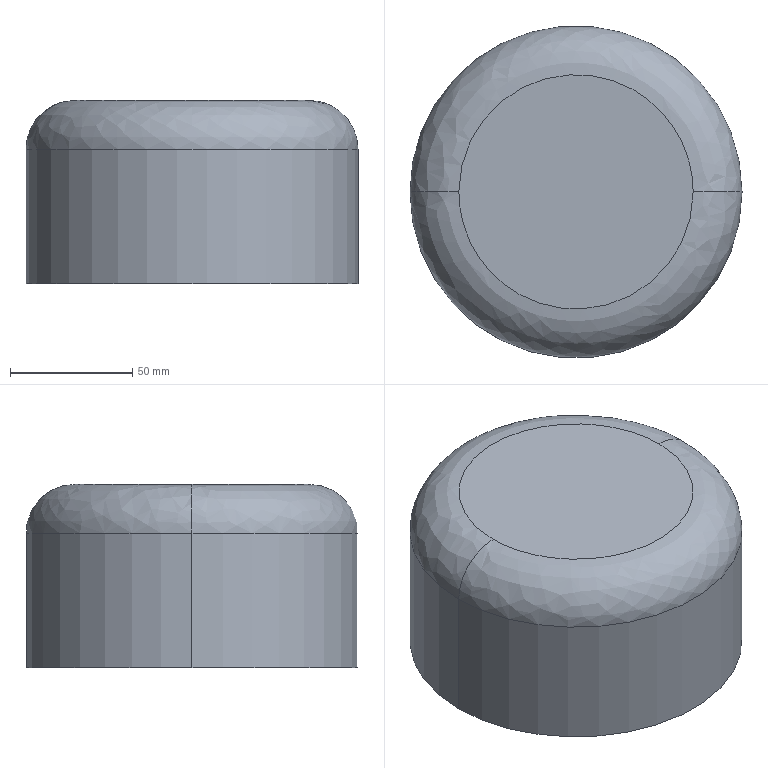Part | SolidWorks | features BaseBody 1 | 1 solid | 11 faces | box 136 x 136 x 75 mm | volume 33898 mm3 | spline 4 | cylinder 4 | plane 3 | commonest cylinder face diameters 134.4 x2 136 x2
STEP:
#1=CARTESIAN_POINT('',(48.,0.,75.));
#2=VERTEX_POINT('',#1);
#3=CARTESIAN_POINT('',(-48.,0.,75.));
#4=VERTEX_POINT('',#3);
#5=CARTESIAN_POINT('',(48.,0.,75.));
#6=CARTESIAN_POINT('',(48.,-96.,75.));
#7=CARTESIAN_POINT('',(-48.,-96.,75.));
#8=CARTESIAN_POINT('',(-48.,0.,75.));
#9=(BOUNDED_CURVE()B_SPLINE_CURVE(3,(#5,#6,#7,#8),.UNSPECIFIED.,.F.,.F.)B_SPLINE_CURVE_WITH_KNOTS((4,4),(0.,0.5),.UNSPECIFIED.)CURVE()GEOMETRIC_REPRESENTATION_ITEM()RATIONAL_B_SPLINE_CURVE((1.,0.3333,0.3333,1.))REPRESENTATION_ITEM(''));
#10=EDGE_CURVE('',#2,#4,#9,.T.);
#11=ORIENTED_EDGE('',*,*,#10,.T.);
#12=CARTESIAN_POINT('',(-68.,0.,55.));
#13=VERTEX_POINT('',#12);
#14=CARTESIAN_POINT('',(-48.,0.,55.));
#15=DIRECTION('',(0.,-1.,0.));
#16=DIRECTION('',(-1.,0.,0.));
#17=AXIS2_PLACEMENT_3D('',#14,#15,#16);
#18=CIRCLE('',#17,20.);
#19=EDGE_CURVE('',#4,#13,#18,.T.);
#20=ORIENTED_EDGE('',*,*,#19,.T.);
#21=CARTESIAN_POINT('',(68.,0.,55.));
#22=VERTEX_POINT('',#21);
#23=CARTESIAN_POINT('',(0.,0.,55.));
#24=DIRECTION('',(0.,0.,-1.));
#25=DIRECTION('',(-1.,0.,0.));
#26=AXIS2_PLACEMENT_3D('',#23,#24,#25);
#27=CIRCLE('',#26,68.);
#28=EDGE_CURVE('',#22,#13,#27,.T.);
#29=ORIENTED_EDGE('',*,*,#28,.F.);
#30=CARTESIAN_POINT('',(48.,0.,55.));
#31=DIRECTION('',(0.,1.,0.));
#32=DIRECTION('',(1.,0.,0.));
#33=AXIS2_PLACEMENT_3D('',#30,#31,#32);
#34=CIRCLE('',#33,20.);
#35=EDGE_CURVE('',#2,#22,#34,.T.);
#36=ORIENTED_EDGE('',*,*,#35,.F.);
#37=EDGE_LOOP('',(#11,#20,#29,#36));
#38=FACE_OUTER_BOUND('',#37,.T.);
#39=CARTESIAN_POINT('',(-48.,0.,75.));
#40=CARTESIAN_POINT('',(-48.,-96.,75.));
#41=CARTESIAN_POINT('',(48.,-96.,75.));
#42=CARTESIAN_POINT('',(48.,0.,75.));
#43=CARTESIAN_POINT('',(-59.716,0.,75.));
#44=CARTESIAN_POINT('',(-59.716,-119.431,75.));
#45=CARTESIAN_POINT('',(59.716,-119.431,75.));
#46=CARTESIAN_POINT('',(59.716,0.,75.));
#47=CARTESIAN_POINT('',(-68.,0.,66.716));
#48=CARTESIAN_POINT('',(-68.,-136.,66.716));
#49=CARTESIAN_POINT('',(68.,-136.,66.716));
#50=CARTESIAN_POINT('',(68.,0.,66.716));
#51=CARTESIAN_POINT('',(-68.,0.,55.));
#52=CARTESIAN_POINT('',(-68.,-136.,55.));
#53=CARTESIAN_POINT('',(68.,-136.,55.));
#54=CARTESIAN_POINT('',(68.,0.,55.));
#55=(BOUNDED_SURFACE()B_SPLINE_SURFACE(3,3,((#39,#40,#41,#42),(#43,#44,#45,#46),(#47,#48,#49,#50),(#51,#52,#53,#54)),.UNSPECIFIED.,.F.,.F.,.F.)B_SPLINE_SURFACE_WITH_KNOTS((4,4),(4,4),(0.,1.),(0.,1.),.UNSPECIFIED.)GEOMETRIC_REPRESENTATION_ITEM()RATIONAL_B_SPLINE_SURFACE(((1.,0.3333,0.3333,1.),(0.8047,0.2682,0.2682,0.8047),(0.8047,0.2682,0.2682,0.8047),(1.,0.3333,0.3333,1.)))REPRESENTATION_ITEM('')SURFACE());
#56=ADVANCED_FACE('',(#38),#55,.T.);
#57=CARTESIAN_POINT('',(-48.,0.,74.2));
#58=VERTEX_POINT('',#57);
#59=CARTESIAN_POINT('',(48.,0.,74.2));
#60=VERTEX_POINT('',#59);
#61=CARTESIAN_POINT('',(-48.,0.,74.2));
#62=CARTESIAN_POINT('',(-48.,1.468,74.2));
#63=CARTESIAN_POINT('',(-47.9,3.661,74.2));
#64=CARTESIAN_POINT('',(-47.608,6.203,74.2));
#65=CARTESIAN_POINT('',(-47.418,7.47,74.2));
#66=CARTESIAN_POINT('',(-47.312,8.102,74.2));
#67=CARTESIAN_POINT('',(-47.256,8.418,74.2));
#68=CARTESIAN_POINT('',(-47.228,8.576,74.2));
#69=CARTESIAN_POINT('',(-47.215,8.644,74.2));
#70=CARTESIAN_POINT('',(-47.207,8.689,74.2));
#71=CARTESIAN_POINT('',(-47.203,8.71,74.2));
#72=CARTESIAN_POINT('',(-46.915,10.265,74.2));
#73=CARTESIAN_POINT('',(-46.382,12.53,74.2));
#74=CARTESIAN_POINT('',(-45.569,15.118,74.2));
#75=CARTESIAN_POINT('',(-45.115,16.398,74.2));
#76=CARTESIAN_POINT('',(-44.877,17.034,74.2));
#77=CARTESIAN_POINT('',(-44.754,17.352,74.2));
#78=CARTESIAN_POINT('',(-44.701,17.488,74.2));
#79=CARTESIAN_POINT('',(-44.666,17.578,74.2));
#80=CARTESIAN_POINT('',(-44.648,17.621,74.2));
#81=CARTESIAN_POINT('',(-44.033,19.177,74.2));
#82=CARTESIAN_POINT('',(-43.028,21.383,74.2));
#83=CARTESIAN_POINT('',(-41.665,23.857,74.2));
#84=CARTESIAN_POINT('',(-40.936,25.07,74.2));
#85=CARTESIAN_POINT('',(-40.56,25.67,74.2));
#86=CARTESIAN_POINT('',(-40.396,25.926,74.2));
#87=CARTESIAN_POINT('',(-40.286,26.096,74.2));
#88=CARTESIAN_POINT('',(-40.232,26.179,74.2));
#89=CARTESIAN_POINT('',(-38.362,29.04,74.2));
#90=CARTESIAN_POINT('',(-36.285,31.598,74.2));
#91=CARTESIAN_POINT('',(-32.769,35.113,74.2));
#92=CARTESIAN_POINT('',(-30.931,36.771,74.2));
#93=CARTESIAN_POINT('',(-28.646,38.531,74.2));
#94=CARTESIAN_POINT('',(-27.468,39.368,74.2));
#95=CARTESIAN_POINT('',(-26.87,39.776,74.2));
#96=CARTESIAN_POINT('',(-26.612,39.948,74.2));
#97=CARTESIAN_POINT('',(-26.439,40.062,74.2));
#98=CARTESIAN_POINT('',(-26.351,40.12,74.2));
#99=CARTESIAN_POINT('',(-24.908,41.063,74.2));
#100=CARTESIAN_POINT('',(-22.815,42.286,74.2));
#101=CARTESIAN_POINT('',(-20.275,43.522,74.2));
#102=CARTESIAN_POINT('',(-18.98,44.092,74.2));
#103=CARTESIAN_POINT('',(-18.326,44.365,74.2));
#104=CARTESIAN_POINT('',(-17.998,44.498,74.2));
#105=CARTESIAN_POINT('',(-17.857,44.555,74.2));
#106=CARTESIAN_POINT('',(-17.763,44.592,74.2));
#107=CARTESIAN_POINT('',(-17.714,44.612,74.2));
#108=CARTESIAN_POINT('',(-16.221,45.203,74.2));
#109=CARTESIAN_POINT('',(-14.019,45.954,74.2));
#110=CARTESIAN_POINT('',(-11.395,46.64,74.2));
#111=CARTESIAN_POINT('',(-10.069,46.935,74.2));
#112=CARTESIAN_POINT('',(-9.403,47.071,74.2));
#113=CARTESIAN_POINT('',(-9.069,47.136,74.2));
#114=CARTESIAN_POINT('',(-8.902,47.167,74.2));
#115=CARTESIAN_POINT('',(-8.83,47.181,74.2));
#116=CARTESIAN_POINT('',(-8.782,47.19,74.2));
#117=CARTESIAN_POINT('',(-8.757,47.194,74.2));
#118=CARTESIAN_POINT('',(-5.847,47.733,74.2));
#119=CARTESIAN_POINT('',(-2.936,48.,74.2));
#120=CARTESIAN_POINT('',(1.468,48.,74.2));
#121=CARTESIAN_POINT('',(3.661,47.9,74.2));
#122=CARTESIAN_POINT('',(6.203,47.608,74.2));
#123=CARTESIAN_POINT('',(7.47,47.418,74.2));
#124=CARTESIAN_POINT('',(8.102,47.312,74.2));
#125=CARTESIAN_POINT('',(8.418,47.256,74.2));
#126=CARTESIAN_POINT('',(8.576,47.228,74.2));
#127=CARTESIAN_POINT('',(8.644,47.215,74.2));
#128=CARTESIAN_POINT('',(8.689,47.207,74.2));
#129=CARTESIAN_POINT('',(8.71,47.203,74.2));
#130=CARTESIAN_POINT('',(10.265,46.915,74.2));
#131=CARTESIAN_POINT('',(12.53,46.382,74.2));
#132=CARTESIAN_POINT('',(15.118,45.569,74.2));
#133=CARTESIAN_POINT('',(16.398,45.115,74.2));
#134=CARTESIAN_POINT('',(17.034,44.877,74.2));
#135=CARTESIAN_POINT('',(17.352,44.754,74.2));
#136=CARTESIAN_POINT('',(17.488,44.701,74.2));
#137=CARTESIAN_POINT('',(17.578,44.666,74.2));
#138=CARTESIAN_POINT('',(17.621,44.648,74.2));
#139=CARTESIAN_POINT('',(19.177,44.033,74.2));
#140=CARTESIAN_POINT('',(21.383,43.028,74.2));
#141=CARTESIAN_POINT('',(23.857,41.665,74.2));
#142=CARTESIAN_POINT('',(25.07,40.936,74.2));
#143=CARTESIAN_POINT('',(25.67,40.56,74.2));
#144=CARTESIAN_POINT('',(25.926,40.396,74.2));
#145=CARTESIAN_POINT('',(26.096,40.286,74.2));
#146=CARTESIAN_POINT('',(26.179,40.232,74.2));
#147=CARTESIAN_POINT('',(29.04,38.362,74.2));
#148=CARTESIAN_POINT('',(31.598,36.285,74.2));
#149=CARTESIAN_POINT('',(35.113,32.769,74.2));
#150=CARTESIAN_POINT('',(36.771,30.931,74.2));
#151=CARTESIAN_POINT('',(38.531,28.646,74.2));
#152=CARTESIAN_POINT('',(39.368,27.468,74.2));
#153=CARTESIAN_POINT('',(39.776,26.87,74.2));
#154=CARTESIAN_POINT('',(39.948,26.612,74.2));
#155=CARTESIAN_POINT('',(40.062,26.439,74.2));
#156=CARTESIAN_POINT('',(40.12,26.351,74.2));
#157=CARTESIAN_POINT('',(41.063,24.908,74.2));
#158=CARTESIAN_POINT('',(42.286,22.815,74.2));
#159=CARTESIAN_POINT('',(43.522,20.275,74.2));
#160=CARTESIAN_POINT('',(44.092,18.98,74.2));
#161=CARTESIAN_POINT('',(44.365,18.326,74.2));
#162=CARTESIAN_POINT('',(44.498,17.998,74.2));
#163=CARTESIAN_POINT('',(44.555,17.857,74.2));
#164=CARTESIAN_POINT('',(44.592,17.763,74.2));
#165=CARTESIAN_POINT('',(44.612,17.714,74.2));
#166=CARTESIAN_POINT('',(45.203,16.221,74.2));
#167=CARTESIAN_POINT('',(45.954,14.019,74.2));
#168=CARTESIAN_POINT('',(46.64,11.395,74.2));
#169=CARTESIAN_POINT('',(46.935,10.069,74.2));
#170=CARTESIAN_POINT('',(47.071,9.403,74.2));
#171=CARTESIAN_POINT('',(47.136,9.069,74.2));
#172=CARTESIAN_POINT('',(47.167,8.902,74.2));
#173=CARTESIAN_POINT('',(47.181,8.83,74.2));
#174=CARTESIAN_POINT('',(47.19,8.782,74.2));
#175=CARTESIAN_POINT('',(47.194,8.757,74.2));
#176=CARTESIAN_POINT('',(47.733,5.847,74.2));
#177=CARTESIAN_POINT('',(48.,2.936,74.2));
#178=CARTESIAN_POINT('',(48.,0.,74.2));
#179=B_SPLINE_CURVE_WITH_KNOTS('',3,(#61,#62,#63,#64,#65,#66,#67,#68,#69,#70,#71,#72,#73,#74,#75,#76,#77,#78,#79,#80,#81,#82,#83,#84,#85,#86,#87,#88,#89,#90,#91,#92,#93,#94,#95,#96,#97,#98,#99,#100,#101,#102,#103,#104,#105,#106,#107,#108,#109,#110,#111,#112,#113,#114,#115,#116,#117,#118,#119,#120,#121,#122,#123,#124,#125,#126,#127,#128,#129,#130,#131,#132,#133,#134,#135,#136,#137,#138,#139,#140,#141,#142,#143,#144,#145,#146,#147,#148,#149,#150,#151,#152,#153,#154,#155,#156,#157,#158,#159,#160,#161,#162,#163,#164,#165,#166,#167,#168,#169,#170,#171,#172,#173,#174,#175,#176,#177,#178),.UNSPECIFIED.,.F.,.F.,(4,1,1,1,1,1,1,2,2,1,1,1,1,1,2,2,1,1,1,1,2,2,2,1,1,1,1,2,2,1,1,1,1,1,2,2,1,1,1,1,1,1,2,2,2,1,1,1,1,1,1,2,2,1,1,1,1,1,2,2,1,1,1,1,2,2,2,1,1,1,1,2,2,1,1,1,1,1,2,2,1,1,1,1,1,1,2,2,4),(0.5,0.5156,0.5234,0.5273,0.5293,0.5303,0.5308,0.531,0.5313,0.5469,0.5547,0.5586,0.5605,0.5615,0.562,0.5625,0.5781,0.5859,0.5898,0.5918,0.5928,0.5938,0.625,0.6406,0.6484,0.6523,0.6543,0.6553,0.6562,0.6719,0.6797,0.6836,0.6855,0.6865,0.687,0.6875,0.7031,0.7109,0.7148,0.7168,0.7178,0.7183,0.7185,0.7187,0.75,0.7656,0.7734,0.7773,0.7793,0.7803,0.7808,0.781,0.7813,0.7969,0.8047,0.8086,0.8105,0.8115,0.812,0.8125,0.8281,0.8359,0.8398,0.8418,0.8428,0.8438,0.875,0.8906,0.8984,0.9023,0.9043,0.9053,0.9063,0.9219,0.9297,0.9336,0.9355,0.9365,0.937,0.9375,0.9531,0.9609,0.9648,0.9668,0.9678,0.9683,0.9685,0.9688,1.),.UNSPECIFIED.);
#180=EDGE_CURVE('',#58,#60,#179,.T.);
#181=ORIENTED_EDGE('',*,*,#180,.F.);
#182=CARTESIAN_POINT('',(-67.2,0.,55.));
#183=VERTEX_POINT('',#182);
#184=CARTESIAN_POINT('',(-48.,0.,55.));
#185=DIRECTION('',(0.,-1.,0.));
#186=DIRECTION('',(-1.,0.,0.));
#187=AXIS2_PLACEMENT_3D('',#184,#185,#186);
#188=CIRCLE('',#187,19.2);
#189=EDGE_CURVE('',#58,#183,#188,.T.);
#190=ORIENTED_EDGE('',*,*,#189,.T.);
#191=CARTESIAN_POINT('',(67.2,0.,55.));
#192=VERTEX_POINT('',#191);
#193=CARTESIAN_POINT('',(0.,0.,55.));
#194=DIRECTION('',(0.,0.,-1.));
#195=DIRECTION('',(-1.,0.,0.));
#196=AXIS2_PLACEMENT_3D('',#193,#194,#195);
#197=CIRCLE('',#196,67.2);
#198=EDGE_CURVE('',#183,#192,#197,.T.);
#199=ORIENTED_EDGE('',*,*,#198,.T.);
#200=CARTESIAN_POINT('',(48.,0.,55.));
#201=DIRECTION('',(0.,1.,0.));
#202=DIRECTION('',(1.,0.,0.));
#203=AXIS2_PLACEMENT_3D('',#200,#201,#202);
#204=CIRCLE('',#203,19.2);
#205=EDGE_CURVE('',#60,#192,#204,.T.);
#206=ORIENTED_EDGE('',*,*,#205,.F.);
#207=EDGE_LOOP('',(#181,#190,#199,#206));
#208=FACE_OUTER_BOUND('',#207,.T.);
#209=CARTESIAN_POINT('',(48.,0.,74.2));
#210=CARTESIAN_POINT('',(48.,96.,74.2));
#211=CARTESIAN_POINT('',(-48.,96.,74.2));
#212=CARTESIAN_POINT('',(-48.,0.,74.2));
#213=CARTESIAN_POINT('',(59.247,0.,74.2));
#214=CARTESIAN_POINT('',(59.247,118.494,74.2));
#215=CARTESIAN_POINT('',(-59.247,118.494,74.2));
#216=CARTESIAN_POINT('',(-59.247,0.,74.2));
#217=CARTESIAN_POINT('',(67.2,0.,66.247));
#218=CARTESIAN_POINT('',(67.2,134.4,66.247));
#219=CARTESIAN_POINT('',(-67.2,134.4,66.247));
#220=CARTESIAN_POINT('',(-67.2,0.,66.247));
#221=CARTESIAN_POINT('',(67.2,0.,55.));
#222=CARTESIAN_POINT('',(67.2,134.4,55.));
#223=CARTESIAN_POINT('',(-67.2,134.4,55.));
#224=CARTESIAN_POINT('',(-67.2,0.,55.));
#225=(BOUNDED_SURFACE()B_SPLINE_SURFACE(3,3,((#209,#210,#211,#212),(#213,#214,#215,#216),(#217,#218,#219,#220),(#221,#222,#223,#224)),.UNSPECIFIED.,.F.,.F.,.F.)B_SPLINE_SURFACE_WITH_KNOTS((4,4),(4,4),(0.,1.),(0.,1.),.UNSPECIFIED.)GEOMETRIC_REPRESENTATION_ITEM()RATIONAL_B_SPLINE_SURFACE(((1.,0.3333,0.3333,1.),(0.8047,0.2682,0.2682,0.8047),(0.8047,0.2682,0.2682,0.8047),(1.,0.3333,0.3333,1.)))REPRESENTATION_ITEM('')SURFACE());
#226=ADVANCED_FACE('',(#208),#225,.F.);
#227=CARTESIAN_POINT('',(0.,0.,55.));
#228=DIRECTION('',(0.,0.,-1.));
#229=DIRECTION('',(-1.,0.,0.));
#230=AXIS2_PLACEMENT_3D('',#227,#228,#229);
#231=CIRCLE('',#230,68.);
#232=EDGE_CURVE('',#13,#22,#231,.T.);
#233=ORIENTED_EDGE('',*,*,#232,.T.);
#234=CARTESIAN_POINT('',(68.,0.,0.));
#235=VERTEX_POINT('',#234);
#236=CARTESIAN_POINT('',(68.,0.,75.));
#237=DIRECTION('',(0.,0.,-1.));
#238=VECTOR('',#237,1000.);
#239=LINE('',#236,#238);
#240=EDGE_CURVE('',#22,#235,#239,.T.);
#241=ORIENTED_EDGE('',*,*,#240,.T.);
#242=CARTESIAN_POINT('',(-68.,0.,0.));
#243=VERTEX_POINT('',#242);
#244=CARTESIAN_POINT('',(0.,0.,0.));
#245=DIRECTION('',(0.,0.,1.));
#246=DIRECTION('',(-1.,0.,0.));
#247=AXIS2_PLACEMENT_3D('',#244,#245,#246);
#248=CIRCLE('',#247,68.);
#249=EDGE_CURVE('',#235,#243,#248,.T.);
#250=ORIENTED_EDGE('',*,*,#249,.T.);
#251=CARTESIAN_POINT('',(-68.,0.,75.));
#252=DIRECTION('',(0.,0.,-1.));
#253=VECTOR('',#252,1000.);
#254=LINE('',#251,#253);
#255=EDGE_CURVE('',#13,#243,#254,.T.);
#256=ORIENTED_EDGE('',*,*,#255,.F.);
#257=EDGE_LOOP('',(#233,#241,#250,#256));
#258=FACE_OUTER_BOUND('',#257,.T.);
#259=CARTESIAN_POINT('',(0.,0.,75.));
#260=DIRECTION('',(0.,0.,-1.));
#261=DIRECTION('',(-1.,0.,0.));
#262=AXIS2_PLACEMENT_3D('',#259,#260,#261);
#263=CYLINDRICAL_SURFACE('',#262,68.);
#264=ADVANCED_FACE('',(#258),#263,.T.);
#265=CARTESIAN_POINT('',(0.,0.,55.));
#266=DIRECTION('',(0.,0.,-1.));
#267=DIRECTION('',(-1.,0.,0.));
#268=AXIS2_PLACEMENT_3D('',#265,#266,#267);
#269=CIRCLE('',#268,67.2);
#270=EDGE_CURVE('',#192,#183,#269,.T.);
#271=ORIENTED_EDGE('',*,*,#270,.F.);
#272=CARTESIAN_POINT('',(67.2,0.,0.));
#273=VERTEX_POINT('',#272);
#274=CARTESIAN_POINT('',(67.2,0.,75.));
#275=DIRECTION('',(0.,0.,-1.));
#276=VECTOR('',#275,1000.);
#277=LINE('',#274,#276);
#278=EDGE_CURVE('',#192,#273,#277,.T.);
#279=ORIENTED_EDGE('',*,*,#278,.T.);
#280=CARTESIAN_POINT('',(-67.2,0.,0.));
#281=VERTEX_POINT('',#280);
#282=CARTESIAN_POINT('',(0.,0.,0.));
#283=DIRECTION('',(0.,0.,-1.));
#284=DIRECTION('',(-1.,0.,0.));
#285=AXIS2_PLACEMENT_3D('',#282,#283,#284);
#286=CIRCLE('',#285,67.2);
#287=EDGE_CURVE('',#273,#281,#286,.T.);
#288=ORIENTED_EDGE('',*,*,#287,.T.);
#289=CARTESIAN_POINT('',(-67.2,0.,75.));
#290=DIRECTION('',(0.,0.,-1.));
#291=VECTOR('',#290,1000.);
#292=LINE('',#289,#291);
#293=EDGE_CURVE('',#183,#281,#292,.T.);
#294=ORIENTED_EDGE('',*,*,#293,.F.);
#295=EDGE_LOOP('',(#271,#279,#288,#294));
#296=FACE_OUTER_BOUND('',#295,.T.);
#297=CARTESIAN_POINT('',(0.,0.,75.));
#298=DIRECTION('',(0.,0.,-1.));
#299=DIRECTION('',(-1.,0.,0.));
#300=AXIS2_PLACEMENT_3D('',#297,#298,#299);
#301=CYLINDRICAL_SURFACE('',#300,67.2);
#302=ADVANCED_FACE('',(#296),#301,.F.);
#303=ORIENTED_EDGE('',*,*,#240,.F.);
#304=ORIENTED_EDGE('',*,*,#28,.T.);
#305=ORIENTED_EDGE('',*,*,#255,.T.);
#306=CARTESIAN_POINT('',(0.,0.,0.));
#307=DIRECTION('',(0.,0.,1.));
#308=DIRECTION('',(-1.,0.,0.));
#309=AXIS2_PLACEMENT_3D('',#306,#307,#308);
#310=CIRCLE('',#309,68.);
#311=EDGE_CURVE('',#243,#235,#310,.T.);
#312=ORIENTED_EDGE('',*,*,#311,.T.);
#313=EDGE_LOOP('',(#303,#304,#305,#312));
#314=FACE_OUTER_BOUND('',#313,.T.);
#315=CARTESIAN_POINT('',(0.,0.,75.));
#316=DIRECTION('',(0.,0.,-1.));
#317=DIRECTION('',(-1.,0.,0.));
#318=AXIS2_PLACEMENT_3D('',#315,#316,#317);
#319=CYLINDRICAL_SURFACE('',#318,68.);
#320=ADVANCED_FACE('',(#314),#319,.T.);
#321=ORIENTED_EDGE('',*,*,#311,.F.);
#322=ORIENTED_EDGE('',*,*,#249,.F.);
#323=EDGE_LOOP('',(#321,#322));
#324=FACE_OUTER_BOUND('',#323,.T.);
#325=CARTESIAN_POINT('',(0.,0.,0.));
#326=DIRECTION('',(0.,0.,-1.));
#327=DIRECTION('',(-1.,0.,0.));
#328=AXIS2_PLACEMENT_3D('',#325,#326,#327);
#329=CIRCLE('',#328,67.2);
#330=EDGE_CURVE('',#281,#273,#329,.T.);
#331=ORIENTED_EDGE('',*,*,#330,.F.);
#332=ORIENTED_EDGE('',*,*,#287,.F.);
#333=EDGE_LOOP('',(#331,#332));
#334=FACE_BOUND('',#333,.T.);
#335=CARTESIAN_POINT('',(0.,0.,0.));
#336=DIRECTION('',(0.,0.,1.));
#337=DIRECTION('',(1.,0.,0.));
#338=AXIS2_PLACEMENT_3D('',#335,#336,#337);
#339=PLANE('',#338);
#340=ADVANCED_FACE('',(#324,#334),#339,.F.);
#341=ORIENTED_EDGE('',*,*,#19,.F.);
#342=CARTESIAN_POINT('',(-48.,0.,75.));
#343=CARTESIAN_POINT('',(-48.,96.,75.));
#344=CARTESIAN_POINT('',(48.,96.,75.));
#345=CARTESIAN_POINT('',(48.,0.,75.));
#346=(BOUNDED_CURVE()B_SPLINE_CURVE(3,(#342,#343,#344,#345),.UNSPECIFIED.,.F.,.F.)B_SPLINE_CURVE_WITH_KNOTS((4,4),(0.5,1.),.UNSPECIFIED.)CURVE()GEOMETRIC_REPRESENTATION_ITEM()RATIONAL_B_SPLINE_CURVE((1.,0.3333,0.3333,1.))REPRESENTATION_ITEM(''));
#347=EDGE_CURVE('',#4,#2,#346,.T.);
#348=ORIENTED_EDGE('',*,*,#347,.T.);
#349=ORIENTED_EDGE('',*,*,#35,.T.);
#350=ORIENTED_EDGE('',*,*,#232,.F.);
#351=EDGE_LOOP('',(#341,#348,#349,#350));
#352=FACE_OUTER_BOUND('',#351,.T.);
#353=CARTESIAN_POINT('',(48.,0.,75.));
#354=CARTESIAN_POINT('',(48.,96.,75.));
#355=CARTESIAN_POINT('',(-48.,96.,75.));
#356=CARTESIAN_POINT('',(-48.,0.,75.));
#357=CARTESIAN_POINT('',(59.716,0.,75.));
#358=CARTESIAN_POINT('',(59.716,119.431,75.));
#359=CARTESIAN_POINT('',(-59.716,119.431,75.));
#360=CARTESIAN_POINT('',(-59.716,0.,75.));
#361=CARTESIAN_POINT('',(68.,0.,66.716));
#362=CARTESIAN_POINT('',(68.,136.,66.716));
#363=CARTESIAN_POINT('',(-68.,136.,66.716));
#364=CARTESIAN_POINT('',(-68.,0.,66.716));
#365=CARTESIAN_POINT('',(68.,0.,55.));
#366=CARTESIAN_POINT('',(68.,136.,55.));
#367=CARTESIAN_POINT('',(-68.,136.,55.));
#368=CARTESIAN_POINT('',(-68.,0.,55.));
#369=(BOUNDED_SURFACE()B_SPLINE_SURFACE(3,3,((#353,#354,#355,#356),(#357,#358,#359,#360),(#361,#362,#363,#364),(#365,#366,#367,#368)),.UNSPECIFIED.,.F.,.F.,.F.)B_SPLINE_SURFACE_WITH_KNOTS((4,4),(4,4),(0.,1.),(0.,1.),.UNSPECIFIED.)GEOMETRIC_REPRESENTATION_ITEM()RATIONAL_B_SPLINE_SURFACE(((1.,0.3333,0.3333,1.),(0.8047,0.2682,0.2682,0.8047),(0.8047,0.2682,0.2682,0.8047),(1.,0.3333,0.3333,1.)))REPRESENTATION_ITEM('')SURFACE());
#370=ADVANCED_FACE('',(#352),#369,.T.);
#371=ORIENTED_EDGE('',*,*,#278,.F.);
#372=ORIENTED_EDGE('',*,*,#198,.F.);
#373=ORIENTED_EDGE('',*,*,#293,.T.);
#374=ORIENTED_EDGE('',*,*,#330,.T.);
#375=EDGE_LOOP('',(#371,#372,#373,#374));
#376=FACE_OUTER_BOUND('',#375,.T.);
#377=CARTESIAN_POINT('',(0.,0.,75.));
#378=DIRECTION('',(0.,0.,-1.));
#379=DIRECTION('',(-1.,0.,0.));
#380=AXIS2_PLACEMENT_3D('',#377,#378,#379);
#381=CYLINDRICAL_SURFACE('',#380,67.2);
#382=ADVANCED_FACE('',(#376),#381,.F.);
#383=ORIENTED_EDGE('',*,*,#10,.F.);
#384=ORIENTED_EDGE('',*,*,#347,.F.);
#385=EDGE_LOOP('',(#383,#384));
#386=FACE_OUTER_BOUND('',#385,.T.);
#387=CARTESIAN_POINT('',(0.,0.,75.));
#388=DIRECTION('',(0.,0.,1.));
#389=DIRECTION('',(1.,0.,0.));
#390=AXIS2_PLACEMENT_3D('',#387,#388,#389);
#391=PLANE('',#390);
#392=ADVANCED_FACE('',(#386),#391,.T.);
#393=ORIENTED_EDGE('',*,*,#189,.F.);
#394=CARTESIAN_POINT('',(48.,0.,74.2));
#395=CARTESIAN_POINT('',(48.,-1.468,74.2));
#396=CARTESIAN_POINT('',(47.9,-3.661,74.2));
#397=CARTESIAN_POINT('',(47.608,-6.203,74.2));
#398=CARTESIAN_POINT('',(47.418,-7.47,74.2));
#399=CARTESIAN_POINT('',(47.312,-8.102,74.2));
#400=CARTESIAN_POINT('',(47.256,-8.418,74.2));
#401=CARTESIAN_POINT('',(47.228,-8.576,74.2));
#402=CARTESIAN_POINT('',(47.215,-8.644,74.2));
#403=CARTESIAN_POINT('',(47.207,-8.689,74.2));
#404=CARTESIAN_POINT('',(47.203,-8.71,74.2));
#405=CARTESIAN_POINT('',(46.915,-10.265,74.2));
#406=CARTESIAN_POINT('',(46.382,-12.53,74.2));
#407=CARTESIAN_POINT('',(45.569,-15.118,74.2));
#408=CARTESIAN_POINT('',(45.115,-16.398,74.2));
#409=CARTESIAN_POINT('',(44.877,-17.034,74.2));
#410=CARTESIAN_POINT('',(44.754,-17.352,74.2));
#411=CARTESIAN_POINT('',(44.701,-17.488,74.2));
#412=CARTESIAN_POINT('',(44.666,-17.578,74.2));
#413=CARTESIAN_POINT('',(44.648,-17.621,74.2));
#414=CARTESIAN_POINT('',(44.033,-19.177,74.2));
#415=CARTESIAN_POINT('',(43.028,-21.383,74.2));
#416=CARTESIAN_POINT('',(41.665,-23.857,74.2));
#417=CARTESIAN_POINT('',(40.936,-25.07,74.2));
#418=CARTESIAN_POINT('',(40.56,-25.67,74.2));
#419=CARTESIAN_POINT('',(40.396,-25.926,74.2));
#420=CARTESIAN_POINT('',(40.286,-26.096,74.2));
#421=CARTESIAN_POINT('',(40.232,-26.179,74.2));
#422=CARTESIAN_POINT('',(38.362,-29.04,74.2));
#423=CARTESIAN_POINT('',(36.285,-31.598,74.2));
#424=CARTESIAN_POINT('',(32.769,-35.113,74.2));
#425=CARTESIAN_POINT('',(30.931,-36.771,74.2));
#426=CARTESIAN_POINT('',(28.646,-38.531,74.2));
#427=CARTESIAN_POINT('',(27.468,-39.368,74.2));
#428=CARTESIAN_POINT('',(26.87,-39.776,74.2));
#429=CARTESIAN_POINT('',(26.612,-39.948,74.2));
#430=CARTESIAN_POINT('',(26.439,-40.062,74.2));
#431=CARTESIAN_POINT('',(26.351,-40.12,74.2));
#432=CARTESIAN_POINT('',(24.908,-41.063,74.2));
#433=CARTESIAN_POINT('',(22.815,-42.286,74.2));
#434=CARTESIAN_POINT('',(20.275,-43.522,74.2));
#435=CARTESIAN_POINT('',(18.98,-44.092,74.2));
#436=CARTESIAN_POINT('',(18.326,-44.365,74.2));
#437=CARTESIAN_POINT('',(17.998,-44.498,74.2));
#438=CARTESIAN_POINT('',(17.857,-44.555,74.2));
#439=CARTESIAN_POINT('',(17.763,-44.592,74.2));
#440=CARTESIAN_POINT('',(17.714,-44.612,74.2));
#441=CARTESIAN_POINT('',(16.221,-45.203,74.2));
#442=CARTESIAN_POINT('',(14.019,-45.954,74.2));
#443=CARTESIAN_POINT('',(11.395,-46.64,74.2));
#444=CARTESIAN_POINT('',(10.069,-46.935,74.2));
#445=CARTESIAN_POINT('',(9.403,-47.071,74.2));
#446=CARTESIAN_POINT('',(9.069,-47.136,74.2));
#447=CARTESIAN_POINT('',(8.902,-47.167,74.2));
#448=CARTESIAN_POINT('',(8.83,-47.181,74.2));
#449=CARTESIAN_POINT('',(8.782,-47.19,74.2));
#450=CARTESIAN_POINT('',(8.757,-47.194,74.2));
#451=CARTESIAN_POINT('',(5.847,-47.733,74.2));
#452=CARTESIAN_POINT('',(2.936,-48.,74.2));
#453=CARTESIAN_POINT('',(-1.468,-48.,74.2));
#454=CARTESIAN_POINT('',(-3.661,-47.9,74.2));
#455=CARTESIAN_POINT('',(-6.203,-47.608,74.2));
#456=CARTESIAN_POINT('',(-7.47,-47.418,74.2));
#457=CARTESIAN_POINT('',(-8.102,-47.312,74.2));
#458=CARTESIAN_POINT('',(-8.418,-47.256,74.2));
#459=CARTESIAN_POINT('',(-8.576,-47.228,74.2));
#460=CARTESIAN_POINT('',(-8.644,-47.215,74.2));
#461=CARTESIAN_POINT('',(-8.689,-47.207,74.2));
#462=CARTESIAN_POINT('',(-8.71,-47.203,74.2));
#463=CARTESIAN_POINT('',(-10.265,-46.915,74.2));
#464=CARTESIAN_POINT('',(-12.53,-46.382,74.2));
#465=CARTESIAN_POINT('',(-15.118,-45.569,74.2));
#466=CARTESIAN_POINT('',(-16.398,-45.115,74.2));
#467=CARTESIAN_POINT('',(-17.034,-44.877,74.2));
#468=CARTESIAN_POINT('',(-17.352,-44.754,74.2));
#469=CARTESIAN_POINT('',(-17.488,-44.701,74.2));
#470=CARTESIAN_POINT('',(-17.578,-44.666,74.2));
#471=CARTESIAN_POINT('',(-17.621,-44.648,74.2));
#472=CARTESIAN_POINT('',(-19.177,-44.033,74.2));
#473=CARTESIAN_POINT('',(-21.383,-43.028,74.2));
#474=CARTESIAN_POINT('',(-23.857,-41.665,74.2));
#475=CARTESIAN_POINT('',(-25.07,-40.936,74.2));
#476=CARTESIAN_POINT('',(-25.67,-40.56,74.2));
#477=CARTESIAN_POINT('',(-25.926,-40.396,74.2));
#478=CARTESIAN_POINT('',(-26.096,-40.286,74.2));
#479=CARTESIAN_POINT('',(-26.179,-40.232,74.2));
#480=CARTESIAN_POINT('',(-29.04,-38.362,74.2));
#481=CARTESIAN_POINT('',(-31.598,-36.285,74.2));
#482=CARTESIAN_POINT('',(-35.113,-32.769,74.2));
#483=CARTESIAN_POINT('',(-36.771,-30.931,74.2));
#484=CARTESIAN_POINT('',(-38.531,-28.646,74.2));
#485=CARTESIAN_POINT('',(-39.368,-27.468,74.2));
#486=CARTESIAN_POINT('',(-39.776,-26.87,74.2));
#487=CARTESIAN_POINT('',(-39.948,-26.612,74.2));
#488=CARTESIAN_POINT('',(-40.062,-26.439,74.2));
#489=CARTESIAN_POINT('',(-40.12,-26.351,74.2));
#490=CARTESIAN_POINT('',(-41.063,-24.908,74.2));
#491=CARTESIAN_POINT('',(-42.286,-22.815,74.2));
#492=CARTESIAN_POINT('',(-43.522,-20.275,74.2));
#493=CARTESIAN_POINT('',(-44.092,-18.98,74.2));
#494=CARTESIAN_POINT('',(-44.365,-18.326,74.2));
#495=CARTESIAN_POINT('',(-44.498,-17.998,74.2));
#496=CARTESIAN_POINT('',(-44.555,-17.857,74.2));
#497=CARTESIAN_POINT('',(-44.592,-17.763,74.2));
#498=CARTESIAN_POINT('',(-44.612,-17.714,74.2));
#499=CARTESIAN_POINT('',(-45.203,-16.221,74.2));
#500=CARTESIAN_POINT('',(-45.954,-14.019,74.2));
#501=CARTESIAN_POINT('',(-46.64,-11.395,74.2));
#502=CARTESIAN_POINT('',(-46.935,-10.069,74.2));
#503=CARTESIAN_POINT('',(-47.071,-9.403,74.2));
#504=CARTESIAN_POINT('',(-47.136,-9.069,74.2));
#505=CARTESIAN_POINT('',(-47.167,-8.902,74.2));
#506=CARTESIAN_POINT('',(-47.181,-8.83,74.2));
#507=CARTESIAN_POINT('',(-47.19,-8.782,74.2));
#508=CARTESIAN_POINT('',(-47.194,-8.757,74.2));
#509=CARTESIAN_POINT('',(-47.733,-5.847,74.2));
#510=CARTESIAN_POINT('',(-48.,-2.936,74.2));
#511=CARTESIAN_POINT('',(-48.,0.,74.2));
#512=B_SPLINE_CURVE_WITH_KNOTS('',3,(#394,#395,#396,#397,#398,#399,#400,#401,#402,#403,#404,#405,#406,#407,#408,#409,#410,#411,#412,#413,#414,#415,#416,#417,#418,#419,#420,#421,#422,#423,#424,#425,#426,#427,#428,#429,#430,#431,#432,#433,#434,#435,#436,#437,#438,#439,#440,#441,#442,#443,#444,#445,#446,#447,#448,#449,#450,#451,#452,#453,#454,#455,#456,#457,#458,#459,#460,#461,#462,#463,#464,#465,#466,#467,#468,#469,#470,#471,#472,#473,#474,#475,#476,#477,#478,#479,#480,#481,#482,#483,#484,#485,#486,#487,#488,#489,#490,#491,#492,#493,#494,#495,#496,#497,#498,#499,#500,#501,#502,#503,#504,#505,#506,#507,#508,#509,#510,#511),.UNSPECIFIED.,.F.,.F.,(4,1,1,1,1,1,1,2,2,1,1,1,1,1,2,2,1,1,1,1,2,2,2,1,1,1,1,2,2,1,1,1,1,1,2,2,1,1,1,1,1,1,2,2,2,1,1,1,1,1,1,2,2,1,1,1,1,1,2,2,1,1,1,1,2,2,2,1,1,1,1,2,2,1,1,1,1,1,2,2,1,1,1,1,1,1,2,2,4),(0.,0.01563,0.02344,0.02734,0.0293,0.03027,0.03076,0.03101,0.03125,0.04688,0.05469,0.05859,0.06055,0.06152,0.06201,0.0625,0.07813,0.08594,0.08984,0.0918,0.09277,0.09375,0.125,0.1406,0.1484,0.1523,0.1543,0.1553,0.1563,0.1719,0.1797,0.1836,0.1855,0.1865,0.187,0.1875,0.2031,0.2109,0.2148,0.2168,0.2178,0.2183,0.2185,0.2188,0.25,0.2656,0.2734,0.2773,0.2793,0.2803,0.2808,0.281,0.2813,0.2969,0.3047,0.3086,0.3105,0.3115,0.312,0.3125,0.3281,0.3359,0.3398,0.3418,0.3428,0.3438,0.375,0.3906,0.3984,0.4023,0.4043,0.4053,0.4063,0.4219,0.4297,0.4336,0.4355,0.4365,0.437,0.4375,0.4531,0.4609,0.4648,0.4668,0.4678,0.4683,0.4685,0.4688,0.5),.UNSPECIFIED.);
#513=EDGE_CURVE('',#60,#58,#512,.T.);
#514=ORIENTED_EDGE('',*,*,#513,.F.);
#515=ORIENTED_EDGE('',*,*,#205,.T.);
#516=ORIENTED_EDGE('',*,*,#270,.T.);
#517=EDGE_LOOP('',(#393,#514,#515,#516));
#518=FACE_OUTER_BOUND('',#517,.T.);
#519=CARTESIAN_POINT('',(-48.,0.,74.2));
#520=CARTESIAN_POINT('',(-48.,-96.,74.2));
#521=CARTESIAN_POINT('',(48.,-96.,74.2));
#522=CARTESIAN_POINT('',(48.,0.,74.2));
#523=CARTESIAN_POINT('',(-59.247,0.,74.2));
#524=CARTESIAN_POINT('',(-59.247,-118.494,74.2));
#525=CARTESIAN_POINT('',(59.247,-118.494,74.2));
#526=CARTESIAN_POINT('',(59.247,0.,74.2));
#527=CARTESIAN_POINT('',(-67.2,0.,66.247));
#528=CARTESIAN_POINT('',(-67.2,-134.4,66.247));
#529=CARTESIAN_POINT('',(67.2,-134.4,66.247));
#530=CARTESIAN_POINT('',(67.2,0.,66.247));
#531=CARTESIAN_POINT('',(-67.2,0.,55.));
#532=CARTESIAN_POINT('',(-67.2,-134.4,55.));
#533=CARTESIAN_POINT('',(67.2,-134.4,55.));
#534=CARTESIAN_POINT('',(67.2,0.,55.));
#535=(BOUNDED_SURFACE()B_SPLINE_SURFACE(3,3,((#519,#520,#521,#522),(#523,#524,#525,#526),(#527,#528,#529,#530),(#531,#532,#533,#534)),.UNSPECIFIED.,.F.,.F.,.F.)B_SPLINE_SURFACE_WITH_KNOTS((4,4),(4,4),(0.,1.),(0.,1.),.UNSPECIFIED.)GEOMETRIC_REPRESENTATION_ITEM()RATIONAL_B_SPLINE_SURFACE(((1.,0.3333,0.3333,1.),(0.8047,0.2682,0.2682,0.8047),(0.8047,0.2682,0.2682,0.8047),(1.,0.3333,0.3333,1.)))REPRESENTATION_ITEM('')SURFACE());
#536=ADVANCED_FACE('',(#518),#535,.F.);
#537=ORIENTED_EDGE('',*,*,#513,.T.);
#538=ORIENTED_EDGE('',*,*,#180,.T.);
#539=EDGE_LOOP('',(#537,#538));
#540=FACE_OUTER_BOUND('',#539,.T.);
#541=CARTESIAN_POINT('',(0.,0.,74.2));
#542=DIRECTION('',(0.,0.,1.));
#543=DIRECTION('',(1.,0.,0.));
#544=AXIS2_PLACEMENT_3D('',#541,#542,#543);
#545=PLANE('',#544);
#546=ADVANCED_FACE('',(#540),#545,.F.);
#547=CLOSED_SHELL('',(#56,#226,#264,#302,#320,#340,#370,#382,#392,#536,#546));
#548=MANIFOLD_SOLID_BREP('',#547);
#549=CARTESIAN_POINT('',(0.,0.,0.));
#550=DIRECTION('',(0.,0.,1.));
#551=DIRECTION('',(1.,0.,0.));
#552=AXIS2_PLACEMENT_3D('',#549,#550,#551);
#553=(LENGTH_UNIT()NAMED_UNIT(*)SI_UNIT(.MILLI.,.METRE.));
#554=UNCERTAINTY_MEASURE_WITH_UNIT(LENGTH_MEASURE(0.00001),#553,'','');
#555=(NAMED_UNIT(*)PLANE_ANGLE_UNIT()SI_UNIT($,.RADIAN.));
#556=(NAMED_UNIT(*)SI_UNIT($,.STERADIAN.)SOLID_ANGLE_UNIT());
#557=(GEOMETRIC_REPRESENTATION_CONTEXT(3)GLOBAL_UNCERTAINTY_ASSIGNED_CONTEXT((#554))GLOBAL_UNIT_ASSIGNED_CONTEXT((#553,#555,#556))REPRESENTATION_CONTEXT('',''));
#558=ADVANCED_BREP_SHAPE_REPRESENTATION('',(#548,#552),#557);